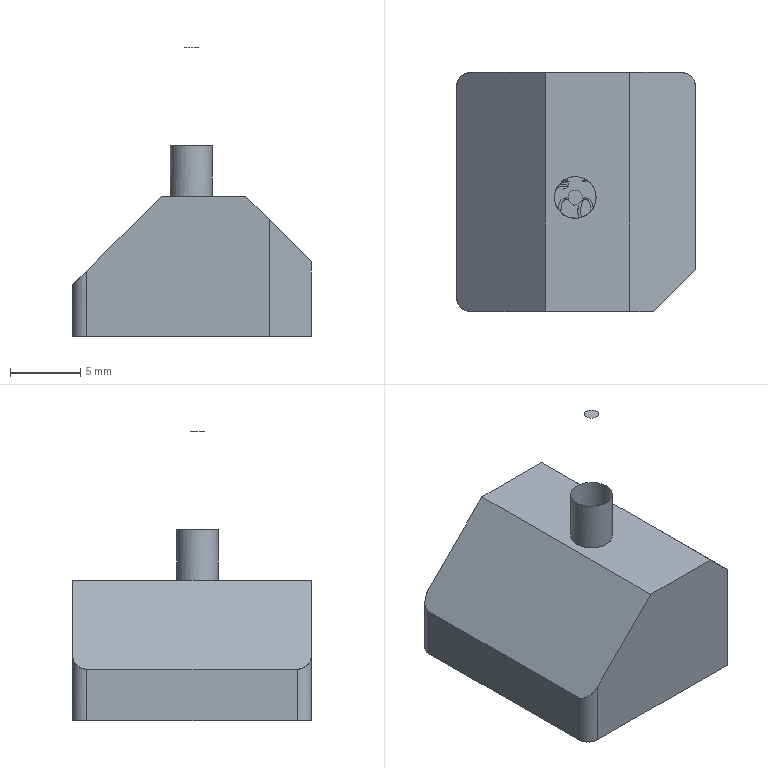CAM job | PowerMill | 3-axis milling, other | part box 17 x 17 x 20.603 mm
Tools:
number,name,type,diameter,tip_radius,length,cutting_length,overhang,flutes,holder,toolpaths_using
1,D10C_1_1_1,end_mill,10.0,0.0,60.0,,21.04,1,D42L35,6
3,D10_1_1_1,end_mill,10.0,0.0,60.0,,20.76,1,D42L35,6
14,D4_1_1,end_mill,4.0,0.0,30.0,,10.76,1,D42L35,2
7,R2_1_1,ball_nosed,4.0,2.0,30.0,,18.2,1,D42L35,1
13,Text_D4_1_1,taper_spherical,4.0,0.3,60.0,,10.88,1,D42L35,2
14,D4_2_1,end_mill,4.0,0.0,30.0,,10.68,1,D42L35,2
7,R2_2_1,ball_nosed,4.0,2.0,30.0,,18.16,1,D42L35,1
Operations:
program,toolpath,strategy,tool,tool_number,tool_diameter,tip_radius,flutes,spindle_rpm,feed_cut,surface_speed_m_min_computed,feed_per_tooth_computed,tolerance,thickness,stepover,stepdown,cut_length,cut_time_min,total_time_min,workplane
30-C01-3-F,精公开粗01-扫面平行-D10C,raster_area_clear,D10C_1_1_1,1,10.0,0.0,1.0,8000.0,10000.0,251.33,1.25,0.03,0.3,6.0,1.0,135.6,0.014,0.0187,
30-C01-3-F,精公开粗01-外形偏置-D10C,offset_area_clear,D10C_1_1_1,1,10.0,0.0,1.0,8000.0,10000.0,251.33,1.25,0.03,0.3,6.0,1.0,3730.801,0.373,0.4409,
30-C01-3-F,精公开粗01-基准台等高-D10C,constantz,D10C_1_1_1,1,10.0,0.0,1.0,8000.0,10000.0,251.33,1.25,0.03,0.07,5.0,0.4,2487.488,0.249,0.2579,
30-C01-3-F,精公基准台01-平坦面平行-D10,raster_area_clear,D10_1_1_1,3,10.0,0.0,1.0,8500.0,600.0,267.04,0.0706,0.005,0.4,5.0,1.0,26.702,0.044,0.06,
30-C01-3-F,精公基准台01-基准面偏置-D10,offset_area_clear,D10_1_1_1,3,10.0,0.0,1.0,8500.0,600.0,267.04,0.0706,0.005,0.4,5.0,1.0,52.31,0.087,0.1051,
30-C01-3-F,精公基准台01-基准台侧光-D10,profile_area_clear,D10_1_1_1,3,10.0,0.0,1.0,8500.0,600.0,267.04,0.0706,0.005,0.0,0.08,1.0,193.234,0.322,0.3859,
30-C01-3-F,精公精光01-等高-D4,constantz,D4_1_1,14,4.0,0.0,1.0,18000.0,2000.0,226.19,0.1111,0.005,-0.055,5.0,0.04,5124.558,2.562,2.999,
30-C01-3-F,精公精光01-平坦面平行-D4,raster_area_clear,D4_1_1,14,4.0,0.0,1.0,18000.0,600.0,226.19,0.0333,0.005,0.395,2.0,1.0,13.326,0.022,0.0319,
30-C01-3-F,精公精光02-平行-R2,raster,R2_1_1,7,4.0,2.0,1.0,18000.0,2000.0,226.19,0.1111,0.005,0.0,0.05,1.0,4684.209,2.342,2.378,
30-C01-3-F,精公刻字01-刻字-Text_D4,pattern,Text_D4_1_1,13,4.0,0.3,1.0,15000.0,1000.0,188.5,0.0667,0.005,0.0,5.0,1.0,8.665,0.009,0.0234,
30-C01-3-R,粗公开粗01-扫面平行-D10C,raster_area_clear,D10C_1_1_1,1,10.0,0.0,1.0,8000.0,10000.0,251.33,1.25,0.03,0.2,6.0,1.0,134.4,0.013,0.0186,
30-C01-3-R,粗公开粗01-外形偏置-D10C,offset_area_clear,D10C_1_1_1,1,10.0,0.0,1.0,8000.0,10000.0,251.33,1.25,0.03,0.2,6.0,1.0,3693.061,0.369,0.4371,
30-C01-3-R,粗公开粗01-基准台等高-D10C,constantz,D10C_1_1_1,1,10.0,0.0,1.0,8000.0,10000.0,251.33,1.25,0.03,0.07,5.0,0.4,2487.488,0.249,0.2579,
30-C01-3-R,粗公基准台01-平坦面平行-D10,raster_area_clear,D10_1_1_1,3,10.0,0.0,1.0,8500.0,600.0,267.04,0.0706,0.01,0.3,5.0,1.0,26.252,0.044,0.0593,
30-C01-3-R,粗公基准台01-基准面偏置-D10,offset_area_clear,D10_1_1_1,3,10.0,0.0,1.0,8500.0,600.0,267.04,0.0706,0.01,0.3,5.0,1.0,52.778,0.088,0.106,
30-C01-3-R,粗公基准台01-基准台侧光-D10,profile_area_clear,D10_1_1_1,3,10.0,0.0,1.0,8500.0,600.0,267.04,0.0706,0.01,0.0,0.08,1.0,193.221,0.322,0.3858,
30-C01-3-R,粗公精光01-等高-D4,constantz,D4_2_1,14,4.0,0.0,1.0,18000.0,2000.0,226.19,0.1111,0.01,-0.155,5.0,0.048,4109.175,2.055,2.417,
30-C01-3-R,粗公精光01-平坦面平行-D4,raster_area_clear,D4_2_1,14,4.0,0.0,1.0,18000.0,600.0,226.19,0.0333,0.01,0.295,2.0,1.0,12.88,0.021,0.0311,
30-C01-3-R,粗公精光02-平行-R2,raster,R2_2_1,7,4.0,2.0,1.0,18000.0,2000.0,226.19,0.1111,0.01,0.0,0.06,1.0,3834.596,1.917,1.953,
30-C01-3-R,粗公刻字01-刻字-Text_D4,pattern,Text_D4_1_1,13,4.0,0.3,1.0,15000.0,1000.0,188.5,0.0667,0.01,0.0,5.0,1.0,8.093,0.008,0.0228,